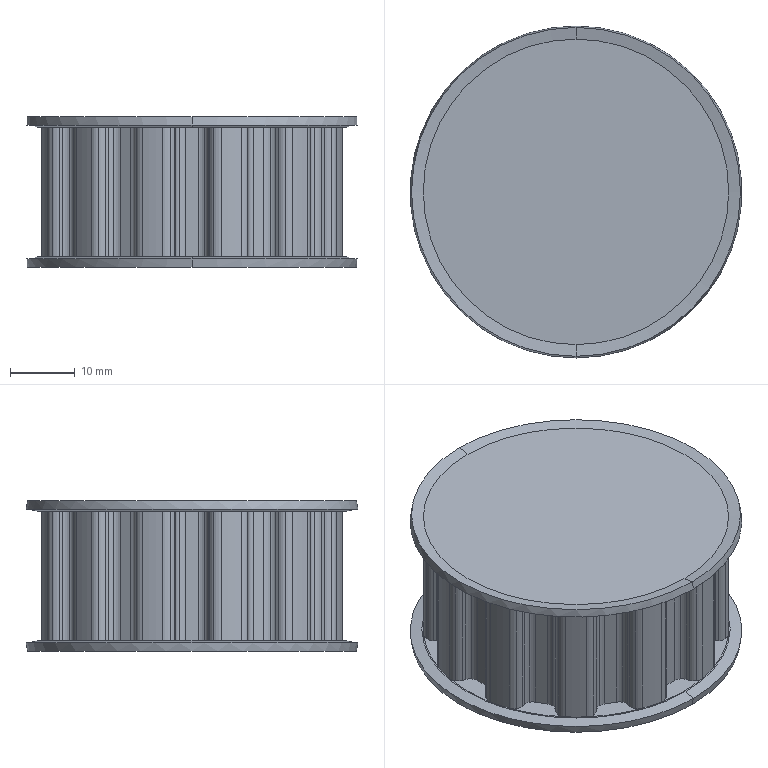Part | SolidWorks | features BaseBody 1 | 1 solid | 186 faces | box 51.203 x 51.203 x 23.179 mm | volume 36269 mm3 | cylinder 108 | plane 62 | cone 12 | torus 4 | commonest cylinder face diameters 3.2 x96 47.139 x12